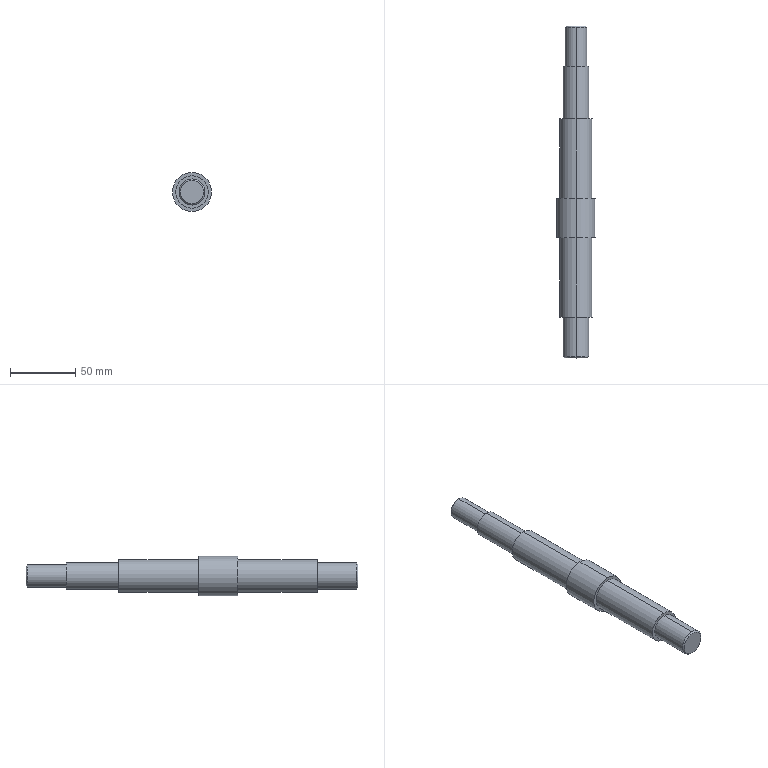Part | STEP file | PN_0021 | 1 solid | 23 faces | box 30 x 255 x 30 mm | volume 110798 mm3 | cylinder 12 | plane 7 | cone 4 | commonest cylinder face diameters 20 x4 25 x4 17 x2 30 x2
STEP:
#1=CARTESIAN_POINT('',(0.,0.,0.));
#2=DIRECTION('',(0.,0.,1.));
#3=DIRECTION('',(1.,0.,0.));
#4=AXIS2_PLACEMENT_3D('',#1,#2,#3);
#5=CARTESIAN_POINT('',(0.,255.,7.5));
#6=VERTEX_POINT('',#5);
#7=CARTESIAN_POINT('',(0.,255.,-7.5));
#8=VERTEX_POINT('',#7);
#9=CARTESIAN_POINT('',(0.,255.,0.));
#10=DIRECTION('',(0.,1.,0.));
#11=DIRECTION('',(0.,0.,1.));
#12=AXIS2_PLACEMENT_3D('',#9,#10,#11);
#13=CIRCLE('',#12,7.5);
#14=CARTESIAN_POINT('',(0.,254.,0.));
#15=DIRECTION('',(0.,-1.,0.));
#16=DIRECTION('',(0.,0.,-1.));
#17=AXIS2_PLACEMENT_3D('',#14,#15,#16);
#18=CONICAL_SURFACE('',#17,8.5,0.7854);
#19=CARTESIAN_POINT('',(3.142,-1.));
#20=DIRECTION('',(-1.,0.));
#21=VECTOR('',#20,1.);
#22=LINE('',#19,#21);
#23=(GEOMETRIC_REPRESENTATION_CONTEXT(2)PARAMETRIC_REPRESENTATION_CONTEXT()REPRESENTATION_CONTEXT('',''));
#24=DEFINITIONAL_REPRESENTATION('',(#22),#23);
#25=PCURVE('',#18,#24);
#26=CARTESIAN_POINT('',(0.,255.,0.));
#27=DIRECTION('',(0.,1.,0.));
#28=DIRECTION('',(0.,0.,1.));
#29=AXIS2_PLACEMENT_3D('',#26,#27,#28);
#30=PLANE('',#29);
#31=CARTESIAN_POINT('',(0.,0.));
#32=DIRECTION('',(1.,0.));
#33=AXIS2_PLACEMENT_2D('',#31,#32);
#34=CIRCLE('',#33,7.5);
#35=(GEOMETRIC_REPRESENTATION_CONTEXT(2)PARAMETRIC_REPRESENTATION_CONTEXT()REPRESENTATION_CONTEXT('',''));
#36=DEFINITIONAL_REPRESENTATION('',(#34),#35);
#37=PCURVE('',#30,#36);
#38=SURFACE_CURVE('',#13,(#25,#37),.PCURVE_S1.);
#39=EDGE_CURVE('',#6,#8,#38,.T.);
#40=ORIENTED_EDGE('',*,*,#39,.F.);
#41=CARTESIAN_POINT('',(0.,254.,8.5));
#42=VERTEX_POINT('',#41);
#43=CARTESIAN_POINT('',(0.,254.,8.5));
#44=DIRECTION('',(0.,-0.7071,0.7071));
#45=VECTOR('',#44,1.);
#46=LINE('',#43,#45);
#47=CARTESIAN_POINT('',(3.142,0.));
#48=DIRECTION('',(0.,1.));
#49=VECTOR('',#48,1.);
#50=LINE('',#47,#49);
#51=(GEOMETRIC_REPRESENTATION_CONTEXT(2)PARAMETRIC_REPRESENTATION_CONTEXT()REPRESENTATION_CONTEXT('',''));
#52=DEFINITIONAL_REPRESENTATION('',(#50),#51);
#53=PCURVE('',#18,#52);
#54=CARTESIAN_POINT('',(0.,254.,0.));
#55=DIRECTION('',(0.,-1.,0.));
#56=DIRECTION('',(0.,0.,-1.));
#57=AXIS2_PLACEMENT_3D('',#54,#55,#56);
#58=CONICAL_SURFACE('',#57,8.5,0.7854);
#59=CARTESIAN_POINT('',(3.142,0.));
#60=DIRECTION('',(0.,1.));
#61=VECTOR('',#60,1.);
#62=LINE('',#59,#61);
#63=(GEOMETRIC_REPRESENTATION_CONTEXT(2)PARAMETRIC_REPRESENTATION_CONTEXT()REPRESENTATION_CONTEXT('',''));
#64=DEFINITIONAL_REPRESENTATION('',(#62),#63);
#65=PCURVE('',#58,#64);
#66=SURFACE_CURVE('',#46,(#53,#65),.PCURVE_S1.);
#67=EDGE_CURVE('',#6,#42,#66,.T.);
#68=ORIENTED_EDGE('',*,*,#67,.T.);
#69=CARTESIAN_POINT('',(0.,254.,-8.5));
#70=VERTEX_POINT('',#69);
#71=CARTESIAN_POINT('',(0.,254.,0.));
#72=DIRECTION('',(0.,-1.,0.));
#73=DIRECTION('',(0.,0.,1.));
#74=AXIS2_PLACEMENT_3D('',#71,#72,#73);
#75=CIRCLE('',#74,8.5);
#76=CARTESIAN_POINT('',(-3.142,0.));
#77=DIRECTION('',(1.,0.));
#78=VECTOR('',#77,1.);
#79=LINE('',#76,#78);
#80=(GEOMETRIC_REPRESENTATION_CONTEXT(2)PARAMETRIC_REPRESENTATION_CONTEXT()REPRESENTATION_CONTEXT('',''));
#81=DEFINITIONAL_REPRESENTATION('',(#79),#80);
#82=PCURVE('',#18,#81);
#83=CARTESIAN_POINT('',(0.,0.,0.));
#84=DIRECTION('',(0.,-1.,0.));
#85=DIRECTION('',(0.,0.,-1.));
#86=AXIS2_PLACEMENT_3D('',#83,#84,#85);
#87=CYLINDRICAL_SURFACE('',#86,8.5);
#88=CARTESIAN_POINT('',(-3.142,-254.));
#89=DIRECTION('',(1.,0.));
#90=VECTOR('',#89,1.);
#91=LINE('',#88,#90);
#92=(GEOMETRIC_REPRESENTATION_CONTEXT(2)PARAMETRIC_REPRESENTATION_CONTEXT()REPRESENTATION_CONTEXT('',''));
#93=DEFINITIONAL_REPRESENTATION('',(#91),#92);
#94=PCURVE('',#87,#93);
#95=SURFACE_CURVE('',#75,(#82,#94),.PCURVE_S1.);
#96=EDGE_CURVE('',#70,#42,#95,.T.);
#97=ORIENTED_EDGE('',*,*,#96,.F.);
#98=CARTESIAN_POINT('',(0.,254.,-8.5));
#99=DIRECTION('',(0.,-0.7071,-0.7071));
#100=VECTOR('',#99,1.);
#101=LINE('',#98,#100);
#102=CARTESIAN_POINT('',(0.,0.));
#103=DIRECTION('',(0.,1.));
#104=VECTOR('',#103,1.);
#105=LINE('',#102,#104);
#106=(GEOMETRIC_REPRESENTATION_CONTEXT(2)PARAMETRIC_REPRESENTATION_CONTEXT()REPRESENTATION_CONTEXT('',''));
#107=DEFINITIONAL_REPRESENTATION('',(#105),#106);
#108=PCURVE('',#18,#107);
#109=CARTESIAN_POINT('',(6.283,0.));
#110=DIRECTION('',(0.,1.));
#111=VECTOR('',#110,1.);
#112=LINE('',#109,#111);
#113=(GEOMETRIC_REPRESENTATION_CONTEXT(2)PARAMETRIC_REPRESENTATION_CONTEXT()REPRESENTATION_CONTEXT('',''));
#114=DEFINITIONAL_REPRESENTATION('',(#112),#113);
#115=PCURVE('',#58,#114);
#116=SURFACE_CURVE('',#101,(#108,#115),.PCURVE_S1.);
#117=EDGE_CURVE('',#8,#70,#116,.T.);
#118=ORIENTED_EDGE('',*,*,#117,.F.);
#119=EDGE_LOOP('',(#40,#68,#97,#118));
#120=FACE_BOUND('',#119,.T.);
#121=ADVANCED_FACE('',(#120),#18,.T.);
#122=CARTESIAN_POINT('',(0.,0.,-9.));
#123=VERTEX_POINT('',#122);
#124=CARTESIAN_POINT('',(0.,0.,9.));
#125=VERTEX_POINT('',#124);
#126=CARTESIAN_POINT('',(0.,0.,0.));
#127=DIRECTION('',(0.,-1.,0.));
#128=DIRECTION('',(0.,0.,-1.));
#129=AXIS2_PLACEMENT_3D('',#126,#127,#128);
#130=CIRCLE('',#129,9.);
#131=CARTESIAN_POINT('',(0.,0.,0.));
#132=DIRECTION('',(0.,1.,0.));
#133=DIRECTION('',(0.,0.,1.));
#134=AXIS2_PLACEMENT_3D('',#131,#132,#133);
#135=CONICAL_SURFACE('',#134,9.,0.7854);
#136=CARTESIAN_POINT('',(3.142,0.));
#137=DIRECTION('',(-1.,0.));
#138=VECTOR('',#137,1.);
#139=LINE('',#136,#138);
#140=(GEOMETRIC_REPRESENTATION_CONTEXT(2)PARAMETRIC_REPRESENTATION_CONTEXT()REPRESENTATION_CONTEXT('',''));
#141=DEFINITIONAL_REPRESENTATION('',(#139),#140);
#142=PCURVE('',#135,#141);
#143=CARTESIAN_POINT('',(0.,0.,0.));
#144=DIRECTION('',(0.,-1.,0.));
#145=DIRECTION('',(0.,0.,-1.));
#146=AXIS2_PLACEMENT_3D('',#143,#144,#145);
#147=PLANE('',#146);
#148=CARTESIAN_POINT('',(0.,0.));
#149=DIRECTION('',(1.,0.));
#150=AXIS2_PLACEMENT_2D('',#148,#149);
#151=CIRCLE('',#150,9.);
#152=(GEOMETRIC_REPRESENTATION_CONTEXT(2)PARAMETRIC_REPRESENTATION_CONTEXT()REPRESENTATION_CONTEXT('',''));
#153=DEFINITIONAL_REPRESENTATION('',(#151),#152);
#154=PCURVE('',#147,#153);
#155=SURFACE_CURVE('',#130,(#142,#154),.PCURVE_S1.);
#156=EDGE_CURVE('',#123,#125,#155,.T.);
#157=ORIENTED_EDGE('',*,*,#156,.F.);
#158=CARTESIAN_POINT('',(0.,1.,-10.));
#159=VERTEX_POINT('',#158);
#160=CARTESIAN_POINT('',(0.,0.,-9.));
#161=DIRECTION('',(0.,0.7071,-0.7071));
#162=VECTOR('',#161,1.);
#163=LINE('',#160,#162);
#164=CARTESIAN_POINT('',(3.142,0.));
#165=DIRECTION('',(0.,1.));
#166=VECTOR('',#165,1.);
#167=LINE('',#164,#166);
#168=(GEOMETRIC_REPRESENTATION_CONTEXT(2)PARAMETRIC_REPRESENTATION_CONTEXT()REPRESENTATION_CONTEXT('',''));
#169=DEFINITIONAL_REPRESENTATION('',(#167),#168);
#170=PCURVE('',#135,#169);
#171=CARTESIAN_POINT('',(0.,0.,0.));
#172=DIRECTION('',(0.,1.,0.));
#173=DIRECTION('',(0.,0.,1.));
#174=AXIS2_PLACEMENT_3D('',#171,#172,#173);
#175=CONICAL_SURFACE('',#174,9.,0.7854);
#176=CARTESIAN_POINT('',(3.142,0.));
#177=DIRECTION('',(0.,1.));
#178=VECTOR('',#177,1.);
#179=LINE('',#176,#178);
#180=(GEOMETRIC_REPRESENTATION_CONTEXT(2)PARAMETRIC_REPRESENTATION_CONTEXT()REPRESENTATION_CONTEXT('',''));
#181=DEFINITIONAL_REPRESENTATION('',(#179),#180);
#182=PCURVE('',#175,#181);
#183=SURFACE_CURVE('',#163,(#170,#182),.PCURVE_S1.);
#184=EDGE_CURVE('',#123,#159,#183,.T.);
#185=ORIENTED_EDGE('',*,*,#184,.T.);
#186=CARTESIAN_POINT('',(0.,1.,10.));
#187=VERTEX_POINT('',#186);
#188=CARTESIAN_POINT('',(0.,1.,0.));
#189=DIRECTION('',(0.,1.,0.));
#190=DIRECTION('',(0.,0.,-1.));
#191=AXIS2_PLACEMENT_3D('',#188,#189,#190);
#192=CIRCLE('',#191,10.);
#193=CARTESIAN_POINT('',(-3.142,1.));
#194=DIRECTION('',(1.,0.));
#195=VECTOR('',#194,1.);
#196=LINE('',#193,#195);
#197=(GEOMETRIC_REPRESENTATION_CONTEXT(2)PARAMETRIC_REPRESENTATION_CONTEXT()REPRESENTATION_CONTEXT('',''));
#198=DEFINITIONAL_REPRESENTATION('',(#196),#197);
#199=PCURVE('',#135,#198);
#200=CARTESIAN_POINT('',(0.,0.,0.));
#201=DIRECTION('',(0.,-1.,0.));
#202=DIRECTION('',(0.,0.,-1.));
#203=AXIS2_PLACEMENT_3D('',#200,#201,#202);
#204=CYLINDRICAL_SURFACE('',#203,10.);
#205=CARTESIAN_POINT('',(6.283,-1.));
#206=DIRECTION('',(-1.,0.));
#207=VECTOR('',#206,1.);
#208=LINE('',#205,#207);
#209=(GEOMETRIC_REPRESENTATION_CONTEXT(2)PARAMETRIC_REPRESENTATION_CONTEXT()REPRESENTATION_CONTEXT('',''));
#210=DEFINITIONAL_REPRESENTATION('',(#208),#209);
#211=PCURVE('',#204,#210);
#212=SURFACE_CURVE('',#192,(#199,#211),.PCURVE_S1.);
#213=EDGE_CURVE('',#187,#159,#212,.T.);
#214=ORIENTED_EDGE('',*,*,#213,.F.);
#215=CARTESIAN_POINT('',(0.,0.,9.));
#216=DIRECTION('',(0.,0.7071,0.7071));
#217=VECTOR('',#216,1.);
#218=LINE('',#215,#217);
#219=CARTESIAN_POINT('',(0.,0.));
#220=DIRECTION('',(0.,1.));
#221=VECTOR('',#220,1.);
#222=LINE('',#219,#221);
#223=(GEOMETRIC_REPRESENTATION_CONTEXT(2)PARAMETRIC_REPRESENTATION_CONTEXT()REPRESENTATION_CONTEXT('',''));
#224=DEFINITIONAL_REPRESENTATION('',(#222),#223);
#225=PCURVE('',#135,#224);
#226=CARTESIAN_POINT('',(6.283,0.));
#227=DIRECTION('',(0.,1.));
#228=VECTOR('',#227,1.);
#229=LINE('',#226,#228);
#230=(GEOMETRIC_REPRESENTATION_CONTEXT(2)PARAMETRIC_REPRESENTATION_CONTEXT()REPRESENTATION_CONTEXT('',''));
#231=DEFINITIONAL_REPRESENTATION('',(#229),#230);
#232=PCURVE('',#175,#231);
#233=SURFACE_CURVE('',#218,(#225,#232),.PCURVE_S1.);
#234=EDGE_CURVE('',#125,#187,#233,.T.);
#235=ORIENTED_EDGE('',*,*,#234,.F.);
#236=EDGE_LOOP('',(#157,#185,#214,#235));
#237=FACE_BOUND('',#236,.T.);
#238=ADVANCED_FACE('',(#237),#135,.T.);
#239=CARTESIAN_POINT('',(0.,31.2,-10.));
#240=VERTEX_POINT('',#239);
#241=CARTESIAN_POINT('',(0.,31.2,10.));
#242=VERTEX_POINT('',#241);
#243=CARTESIAN_POINT('',(0.,31.2,0.));
#244=DIRECTION('',(0.,-1.,0.));
#245=DIRECTION('',(0.,0.,-1.));
#246=AXIS2_PLACEMENT_3D('',#243,#244,#245);
#247=CIRCLE('',#246,10.);
#248=CARTESIAN_POINT('',(0.,-31.2));
#249=DIRECTION('',(1.,0.));
#250=VECTOR('',#249,1.);
#251=LINE('',#248,#250);
#252=(GEOMETRIC_REPRESENTATION_CONTEXT(2)PARAMETRIC_REPRESENTATION_CONTEXT()REPRESENTATION_CONTEXT('',''));
#253=DEFINITIONAL_REPRESENTATION('',(#251),#252);
#254=PCURVE('',#204,#253);
#255=CARTESIAN_POINT('',(10.,31.2,0.));
#256=DIRECTION('',(0.,-1.,0.));
#257=DIRECTION('',(0.,0.,-1.));
#258=AXIS2_PLACEMENT_3D('',#255,#256,#257);
#259=PLANE('',#258);
#260=CARTESIAN_POINT('',(0.,-10.));
#261=DIRECTION('',(1.,0.));
#262=AXIS2_PLACEMENT_2D('',#260,#261);
#263=CIRCLE('',#262,10.);
#264=(GEOMETRIC_REPRESENTATION_CONTEXT(2)PARAMETRIC_REPRESENTATION_CONTEXT()REPRESENTATION_CONTEXT('',''));
#265=DEFINITIONAL_REPRESENTATION('',(#263),#264);
#266=PCURVE('',#259,#265);
#267=SURFACE_CURVE('',#247,(#254,#266),.PCURVE_S1.);
#268=EDGE_CURVE('',#240,#242,#267,.T.);
#269=ORIENTED_EDGE('',*,*,#268,.T.);
#270=CARTESIAN_POINT('',(0.,0.,10.));
#271=DIRECTION('',(0.,-1.,0.));
#272=VECTOR('',#271,1.);
#273=LINE('',#270,#272);
#274=CARTESIAN_POINT('',(3.142,0.));
#275=DIRECTION('',(0.,1.));
#276=VECTOR('',#275,1.);
#277=LINE('',#274,#276);
#278=(GEOMETRIC_REPRESENTATION_CONTEXT(2)PARAMETRIC_REPRESENTATION_CONTEXT()REPRESENTATION_CONTEXT('',''));
#279=DEFINITIONAL_REPRESENTATION('',(#277),#278);
#280=PCURVE('',#204,#279);
#281=CARTESIAN_POINT('',(0.,0.,0.));
#282=DIRECTION('',(0.,-1.,0.));
#283=DIRECTION('',(0.,0.,-1.));
#284=AXIS2_PLACEMENT_3D('',#281,#282,#283);
#285=CYLINDRICAL_SURFACE('',#284,10.);
#286=CARTESIAN_POINT('',(3.142,0.));
#287=DIRECTION('',(0.,1.));
#288=VECTOR('',#287,1.);
#289=LINE('',#286,#288);
#290=(GEOMETRIC_REPRESENTATION_CONTEXT(2)PARAMETRIC_REPRESENTATION_CONTEXT()REPRESENTATION_CONTEXT('',''));
#291=DEFINITIONAL_REPRESENTATION('',(#289),#290);
#292=PCURVE('',#285,#291);
#293=SURFACE_CURVE('',#273,(#280,#292),.PCURVE_S1.);
#294=EDGE_CURVE('',#242,#187,#293,.T.);
#295=ORIENTED_EDGE('',*,*,#294,.T.);
#296=ORIENTED_EDGE('',*,*,#213,.T.);
#297=CARTESIAN_POINT('',(0.,0.,-10.));
#298=DIRECTION('',(0.,-1.,0.));
#299=VECTOR('',#298,1.);
#300=LINE('',#297,#299);
#301=CARTESIAN_POINT('',(0.,0.));
#302=DIRECTION('',(0.,1.));
#303=VECTOR('',#302,1.);
#304=LINE('',#301,#303);
#305=(GEOMETRIC_REPRESENTATION_CONTEXT(2)PARAMETRIC_REPRESENTATION_CONTEXT()REPRESENTATION_CONTEXT('',''));
#306=DEFINITIONAL_REPRESENTATION('',(#304),#305);
#307=PCURVE('',#204,#306);
#308=CARTESIAN_POINT('',(6.283,0.));
#309=DIRECTION('',(0.,1.));
#310=VECTOR('',#309,1.);
#311=LINE('',#308,#310);
#312=(GEOMETRIC_REPRESENTATION_CONTEXT(2)PARAMETRIC_REPRESENTATION_CONTEXT()REPRESENTATION_CONTEXT('',''));
#313=DEFINITIONAL_REPRESENTATION('',(#311),#312);
#314=PCURVE('',#285,#313);
#315=SURFACE_CURVE('',#300,(#307,#314),.PCURVE_S1.);
#316=EDGE_CURVE('',#240,#159,#315,.T.);
#317=ORIENTED_EDGE('',*,*,#316,.F.);
#318=EDGE_LOOP('',(#269,#295,#296,#317));
#319=FACE_BOUND('',#318,.T.);
#320=ADVANCED_FACE('',(#319),#204,.T.);
#321=CARTESIAN_POINT('',(0.,92.5,-12.5));
#322=VERTEX_POINT('',#321);
#323=CARTESIAN_POINT('',(0.,92.5,12.5));
#324=VERTEX_POINT('',#323);
#325=CARTESIAN_POINT('',(0.,92.5,0.));
#326=DIRECTION('',(0.,-1.,0.));
#327=DIRECTION('',(0.,0.,-1.));
#328=AXIS2_PLACEMENT_3D('',#325,#326,#327);
#329=CIRCLE('',#328,12.5);
#330=CARTESIAN_POINT('',(0.,0.,0.));
#331=DIRECTION('',(0.,-1.,0.));
#332=DIRECTION('',(0.,0.,-1.));
#333=AXIS2_PLACEMENT_3D('',#330,#331,#332);
#334=CYLINDRICAL_SURFACE('',#333,12.5);
#335=CARTESIAN_POINT('',(0.,-92.5));
#336=DIRECTION('',(1.,0.));
#337=VECTOR('',#336,1.);
#338=LINE('',#335,#337);
#339=(GEOMETRIC_REPRESENTATION_CONTEXT(2)PARAMETRIC_REPRESENTATION_CONTEXT()REPRESENTATION_CONTEXT('',''));
#340=DEFINITIONAL_REPRESENTATION('',(#338),#339);
#341=PCURVE('',#334,#340);
#342=CARTESIAN_POINT('',(12.5,92.5,0.));
#343=DIRECTION('',(0.,-1.,0.));
#344=DIRECTION('',(0.,0.,-1.));
#345=AXIS2_PLACEMENT_3D('',#342,#343,#344);
#346=PLANE('',#345);
#347=CARTESIAN_POINT('',(0.,-12.5));
#348=DIRECTION('',(1.,0.));
#349=AXIS2_PLACEMENT_2D('',#347,#348);
#350=CIRCLE('',#349,12.5);
#351=(GEOMETRIC_REPRESENTATION_CONTEXT(2)PARAMETRIC_REPRESENTATION_CONTEXT()REPRESENTATION_CONTEXT('',''));
#352=DEFINITIONAL_REPRESENTATION('',(#350),#351);
#353=PCURVE('',#346,#352);
#354=SURFACE_CURVE('',#329,(#341,#353),.PCURVE_S1.);
#355=EDGE_CURVE('',#322,#324,#354,.T.);
#356=ORIENTED_EDGE('',*,*,#355,.T.);
#357=CARTESIAN_POINT('',(0.,31.2,12.5));
#358=VERTEX_POINT('',#357);
#359=CARTESIAN_POINT('',(0.,0.,12.5));
#360=DIRECTION('',(0.,-1.,0.));
#361=VECTOR('',#360,1.);
#362=LINE('',#359,#361);
#363=CARTESIAN_POINT('',(3.142,0.));
#364=DIRECTION('',(0.,1.));
#365=VECTOR('',#364,1.);
#366=LINE('',#363,#365);
#367=(GEOMETRIC_REPRESENTATION_CONTEXT(2)PARAMETRIC_REPRESENTATION_CONTEXT()REPRESENTATION_CONTEXT('',''));
#368=DEFINITIONAL_REPRESENTATION('',(#366),#367);
#369=PCURVE('',#334,#368);
#370=CARTESIAN_POINT('',(0.,0.,0.));
#371=DIRECTION('',(0.,-1.,0.));
#372=DIRECTION('',(0.,0.,-1.));
#373=AXIS2_PLACEMENT_3D('',#370,#371,#372);
#374=CYLINDRICAL_SURFACE('',#373,12.5);
#375=CARTESIAN_POINT('',(3.142,0.));
#376=DIRECTION('',(0.,1.));
#377=VECTOR('',#376,1.);
#378=LINE('',#375,#377);
#379=(GEOMETRIC_REPRESENTATION_CONTEXT(2)PARAMETRIC_REPRESENTATION_CONTEXT()REPRESENTATION_CONTEXT('',''));
#380=DEFINITIONAL_REPRESENTATION('',(#378),#379);
#381=PCURVE('',#374,#380);
#382=SURFACE_CURVE('',#362,(#369,#381),.PCURVE_S1.);
#383=EDGE_CURVE('',#324,#358,#382,.T.);
#384=ORIENTED_EDGE('',*,*,#383,.T.);
#385=CARTESIAN_POINT('',(0.,31.2,-12.5));
#386=VERTEX_POINT('',#385);
#387=CARTESIAN_POINT('',(0.,31.2,0.));
#388=DIRECTION('',(0.,-1.,0.));
#389=DIRECTION('',(0.,0.,-1.));
#390=AXIS2_PLACEMENT_3D('',#387,#388,#389);
#391=CIRCLE('',#390,12.5);
#392=CARTESIAN_POINT('',(0.,-31.2));
#393=DIRECTION('',(1.,0.));
#394=VECTOR('',#393,1.);
#395=LINE('',#392,#394);
#396=(GEOMETRIC_REPRESENTATION_CONTEXT(2)PARAMETRIC_REPRESENTATION_CONTEXT()REPRESENTATION_CONTEXT('',''));
#397=DEFINITIONAL_REPRESENTATION('',(#395),#396);
#398=PCURVE('',#334,#397);
#399=CARTESIAN_POINT('',(0.,-10.));
#400=DIRECTION('',(1.,0.));
#401=AXIS2_PLACEMENT_2D('',#399,#400);
#402=CIRCLE('',#401,12.5);
#403=(GEOMETRIC_REPRESENTATION_CONTEXT(2)PARAMETRIC_REPRESENTATION_CONTEXT()REPRESENTATION_CONTEXT('',''));
#404=DEFINITIONAL_REPRESENTATION('',(#402),#403);
#405=PCURVE('',#259,#404);
#406=SURFACE_CURVE('',#391,(#398,#405),.PCURVE_S1.);
#407=EDGE_CURVE('',#386,#358,#406,.T.);
#408=ORIENTED_EDGE('',*,*,#407,.F.);
#409=CARTESIAN_POINT('',(0.,0.,-12.5));
#410=DIRECTION('',(0.,-1.,0.));
#411=VECTOR('',#410,1.);
#412=LINE('',#409,#411);
#413=CARTESIAN_POINT('',(0.,0.));
#414=DIRECTION('',(0.,1.));
#415=VECTOR('',#414,1.);
#416=LINE('',#413,#415);
#417=(GEOMETRIC_REPRESENTATION_CONTEXT(2)PARAMETRIC_REPRESENTATION_CONTEXT()REPRESENTATION_CONTEXT('',''));
#418=DEFINITIONAL_REPRESENTATION('',(#416),#417);
#419=PCURVE('',#334,#418);
#420=CARTESIAN_POINT('',(6.283,0.));
#421=DIRECTION('',(0.,1.));
#422=VECTOR('',#421,1.);
#423=LINE('',#420,#422);
#424=(GEOMETRIC_REPRESENTATION_CONTEXT(2)PARAMETRIC_REPRESENTATION_CONTEXT()REPRESENTATION_CONTEXT('',''));
#425=DEFINITIONAL_REPRESENTATION('',(#423),#424);
#426=PCURVE('',#374,#425);
#427=SURFACE_CURVE('',#412,(#419,#426),.PCURVE_S1.);
#428=EDGE_CURVE('',#322,#386,#427,.T.);
#429=ORIENTED_EDGE('',*,*,#428,.F.);
#430=EDGE_LOOP('',(#356,#384,#408,#429));
#431=FACE_BOUND('',#430,.T.);
#432=ADVANCED_FACE('',(#431),#334,.T.);
#433=CARTESIAN_POINT('',(0.,122.5,-15.));
#434=VERTEX_POINT('',#433);
#435=CARTESIAN_POINT('',(0.,122.5,15.));
#436=VERTEX_POINT('',#435);
#437=CARTESIAN_POINT('',(0.,122.5,0.));
#438=DIRECTION('',(0.,-1.,0.));
#439=DIRECTION('',(0.,0.,-1.));
#440=AXIS2_PLACEMENT_3D('',#437,#438,#439);
#441=CIRCLE('',#440,15.);
#442=CARTESIAN_POINT('',(0.,0.,0.));
#443=DIRECTION('',(0.,-1.,0.));
#444=DIRECTION('',(0.,0.,-1.));
#445=AXIS2_PLACEMENT_3D('',#442,#443,#444);
#446=CYLINDRICAL_SURFACE('',#445,15.);
#447=CARTESIAN_POINT('',(0.,-122.5));
#448=DIRECTION('',(1.,0.));
#449=VECTOR('',#448,1.);
#450=LINE('',#447,#449);
#451=(GEOMETRIC_REPRESENTATION_CONTEXT(2)PARAMETRIC_REPRESENTATION_CONTEXT()REPRESENTATION_CONTEXT('',''));
#452=DEFINITIONAL_REPRESENTATION('',(#450),#451);
#453=PCURVE('',#446,#452);
#454=CARTESIAN_POINT('',(12.5,122.5,0.));
#455=DIRECTION('',(0.,1.,0.));
#456=DIRECTION('',(0.,0.,1.));
#457=AXIS2_PLACEMENT_3D('',#454,#455,#456);
#458=PLANE('',#457);
#459=CARTESIAN_POINT('',(-15.,-12.5));
#460=CARTESIAN_POINT('',(-15.,13.481));
#461=CARTESIAN_POINT('',(7.5,0.4904));
#462=CARTESIAN_POINT('',(30.,-12.5));
#463=CARTESIAN_POINT('',(7.5,-25.49));
#464=CARTESIAN_POINT('',(-15.,-38.481));
#465=CARTESIAN_POINT('',(-15.,-12.5));
#466=(BOUNDED_CURVE()B_SPLINE_CURVE(2,(#459,#460,#461,#462,#463,#464,#465),.UNSPECIFIED.,.T.,.F.)B_SPLINE_CURVE_WITH_KNOTS((1,2,2,2,2,1),(-2.094,0.,2.094,4.189,6.283,8.378),.UNSPECIFIED.)CURVE()GEOMETRIC_REPRESENTATION_ITEM()RATIONAL_B_SPLINE_CURVE((1.,0.5,1.,0.5,1.,0.5,1.))REPRESENTATION_ITEM(''));
#467=(GEOMETRIC_REPRESENTATION_CONTEXT(2)PARAMETRIC_REPRESENTATION_CONTEXT()REPRESENTATION_CONTEXT('',''));
#468=DEFINITIONAL_REPRESENTATION('',(#466),#467);
#469=PCURVE('',#458,#468);
#470=SURFACE_CURVE('',#441,(#453,#469),.PCURVE_S1.);
#471=EDGE_CURVE('',#434,#436,#470,.T.);
#472=ORIENTED_EDGE('',*,*,#471,.T.);
#473=CARTESIAN_POINT('',(0.,92.5,15.));
#474=VERTEX_POINT('',#473);
#475=CARTESIAN_POINT('',(0.,0.,15.));
#476=DIRECTION('',(0.,-1.,0.));
#477=VECTOR('',#476,1.);
#478=LINE('',#475,#477);
#479=CARTESIAN_POINT('',(3.142,0.));
#480=DIRECTION('',(0.,1.));
#481=VECTOR('',#480,1.);
#482=LINE('',#479,#481);
#483=(GEOMETRIC_REPRESENTATION_CONTEXT(2)PARAMETRIC_REPRESENTATION_CONTEXT()REPRESENTATION_CONTEXT('',''));
#484=DEFINITIONAL_REPRESENTATION('',(#482),#483);
#485=PCURVE('',#446,#484);
#486=CARTESIAN_POINT('',(0.,0.,0.));
#487=DIRECTION('',(0.,-1.,0.));
#488=DIRECTION('',(0.,0.,-1.));
#489=AXIS2_PLACEMENT_3D('',#486,#487,#488);
#490=CYLINDRICAL_SURFACE('',#489,15.);
#491=CARTESIAN_POINT('',(3.142,0.));
#492=DIRECTION('',(0.,1.));
#493=VECTOR('',#492,1.);
#494=LINE('',#491,#493);
#495=(GEOMETRIC_REPRESENTATION_CONTEXT(2)PARAMETRIC_REPRESENTATION_CONTEXT()REPRESENTATION_CONTEXT('',''));
#496=DEFINITIONAL_REPRESENTATION('',(#494),#495);
#497=PCURVE('',#490,#496);
#498=SURFACE_CURVE('',#478,(#485,#497),.PCURVE_S1.);
#499=EDGE_CURVE('',#436,#474,#498,.T.);
#500=ORIENTED_EDGE('',*,*,#499,.T.);
#501=CARTESIAN_POINT('',(0.,92.5,-15.));
#502=VERTEX_POINT('',#501);
#503=CARTESIAN_POINT('',(0.,92.5,0.));
#504=DIRECTION('',(0.,-1.,0.));
#505=DIRECTION('',(0.,0.,-1.));
#506=AXIS2_PLACEMENT_3D('',#503,#504,#505);
#507=CIRCLE('',#506,15.);
#508=CARTESIAN_POINT('',(0.,-92.5));
#509=DIRECTION('',(1.,0.));
#510=VECTOR('',#509,1.);
#511=LINE('',#508,#510);
#512=(GEOMETRIC_REPRESENTATION_CONTEXT(2)PARAMETRIC_REPRESENTATION_CONTEXT()REPRESENTATION_CONTEXT('',''));
#513=DEFINITIONAL_REPRESENTATION('',(#511),#512);
#514=PCURVE('',#446,#513);
#515=CARTESIAN_POINT('',(0.,-12.5));
#516=DIRECTION('',(1.,0.));
#517=AXIS2_PLACEMENT_2D('',#515,#516);
#518=CIRCLE('',#517,15.);
#519=(GEOMETRIC_REPRESENTATION_CONTEXT(2)PARAMETRIC_REPRESENTATION_CONTEXT()REPRESENTATION_CONTEXT('',''));
#520=DEFINITIONAL_REPRESENTATION('',(#518),#519);
#521=PCURVE('',#346,#520);
#522=SURFACE_CURVE('',#507,(#514,#521),.PCURVE_S1.);
#523=EDGE_CURVE('',#502,#474,#522,.T.);
#524=ORIENTED_EDGE('',*,*,#523,.F.);
#525=CARTESIAN_POINT('',(0.,0.,-15.));
#526=DIRECTION('',(0.,-1.,0.));
#527=VECTOR('',#526,1.);
#528=LINE('',#525,#527);
#529=CARTESIAN_POINT('',(0.,0.));
#530=DIRECTION('',(0.,1.));
#531=VECTOR('',#530,1.);
#532=LINE('',#529,#531);
#533=(GEOMETRIC_REPRESENTATION_CONTEXT(2)PARAMETRIC_REPRESENTATION_CONTEXT()REPRESENTATION_CONTEXT('',''));
#534=DEFINITIONAL_REPRESENTATION('',(#532),#533);
#535=PCURVE('',#446,#534);
#536=CARTESIAN_POINT('',(6.283,0.));
#537=DIRECTION('',(0.,1.));
#538=VECTOR('',#537,1.);
#539=LINE('',#536,#538);
#540=(GEOMETRIC_REPRESENTATION_CONTEXT(2)PARAMETRIC_REPRESENTATION_CONTEXT()REPRESENTATION_CONTEXT('',''));
#541=DEFINITIONAL_REPRESENTATION('',(#539),#540);
#542=PCURVE('',#490,#541);
#543=SURFACE_CURVE('',#528,(#535,#542),.PCURVE_S1.);
#544=EDGE_CURVE('',#434,#502,#543,.T.);
#545=ORIENTED_EDGE('',*,*,#544,.F.);
#546=EDGE_LOOP('',(#472,#500,#524,#545));
#547=FACE_BOUND('',#546,.T.);
#548=ADVANCED_FACE('',(#547),#446,.T.);
#549=CARTESIAN_POINT('',(0.,183.8,-12.5));
#550=VERTEX_POINT('',#549);
#551=CARTESIAN_POINT('',(0.,183.8,12.5));
#552=VERTEX_POINT('',#551);
#553=CARTESIAN_POINT('',(0.,183.8,0.));
#554=DIRECTION('',(0.,-1.,0.));
#555=DIRECTION('',(0.,0.,-1.));
#556=AXIS2_PLACEMENT_3D('',#553,#554,#555);
#557=CIRCLE('',#556,12.5);
#558=CARTESIAN_POINT('',(0.,0.,0.));
#559=DIRECTION('',(0.,-1.,0.));
#560=DIRECTION('',(0.,0.,-1.));
#561=AXIS2_PLACEMENT_3D('',#558,#559,#560);
#562=CYLINDRICAL_SURFACE('',#561,12.5);
#563=CARTESIAN_POINT('',(0.,-183.8));
#564=DIRECTION('',(1.,0.));
#565=VECTOR('',#564,1.);
#566=LINE('',#563,#565);
#567=(GEOMETRIC_REPRESENTATION_CONTEXT(2)PARAMETRIC_REPRESENTATION_CONTEXT()REPRESENTATION_CONTEXT('',''));
#568=DEFINITIONAL_REPRESENTATION('',(#566),#567);
#569=PCURVE('',#562,#568);
#570=CARTESIAN_POINT('',(10.,183.8,0.));
#571=DIRECTION('',(0.,1.,0.));
#572=DIRECTION('',(0.,0.,1.));
#573=AXIS2_PLACEMENT_3D('',#570,#571,#572);
#574=PLANE('',#573);
#575=CARTESIAN_POINT('',(-12.5,-10.));
#576=CARTESIAN_POINT('',(-12.5,11.651));
#577=CARTESIAN_POINT('',(6.25,0.8253));
#578=CARTESIAN_POINT('',(25.,-10.));
#579=CARTESIAN_POINT('',(6.25,-20.825));
#580=CARTESIAN_POINT('',(-12.5,-31.651));
#581=CARTESIAN_POINT('',(-12.5,-10.));
#582=(BOUNDED_CURVE()B_SPLINE_CURVE(2,(#575,#576,#577,#578,#579,#580,#581),.UNSPECIFIED.,.T.,.F.)B_SPLINE_CURVE_WITH_KNOTS((1,2,2,2,2,1),(-2.094,0.,2.094,4.189,6.283,8.378),.UNSPECIFIED.)CURVE()GEOMETRIC_REPRESENTATION_ITEM()RATIONAL_B_SPLINE_CURVE((1.,0.5,1.,0.5,1.,0.5,1.))REPRESENTATION_ITEM(''));
#583=(GEOMETRIC_REPRESENTATION_CONTEXT(2)PARAMETRIC_REPRESENTATION_CONTEXT()REPRESENTATION_CONTEXT('',''));
#584=DEFINITIONAL_REPRESENTATION('',(#582),#583);
#585=PCURVE('',#574,#584);
#586=SURFACE_CURVE('',#557,(#569,#585),.PCURVE_S1.);
#587=EDGE_CURVE('',#550,#552,#586,.T.);
#588=ORIENTED_EDGE('',*,*,#587,.T.);
#589=CARTESIAN_POINT('',(0.,122.5,12.5));
#590=VERTEX_POINT('',#589);
#591=CARTESIAN_POINT('',(0.,0.,12.5));
#592=DIRECTION('',(0.,-1.,0.));
#593=VECTOR('',#592,1.);
#594=LINE('',#591,#593);
#595=CARTESIAN_POINT('',(3.142,0.));
#596=DIRECTION('',(0.,1.));
#597=VECTOR('',#596,1.);
#598=LINE('',#595,#597);
#599=(GEOMETRIC_REPRESENTATION_CONTEXT(2)PARAMETRIC_REPRESENTATION_CONTEXT()REPRESENTATION_CONTEXT('',''));
#600=DEFINITIONAL_REPRESENTATION('',(#598),#599);
#601=PCURVE('',#562,#600);
#602=CARTESIAN_POINT('',(0.,0.,0.));
#603=DIRECTION('',(0.,-1.,0.));
#604=DIRECTION('',(0.,0.,-1.));
#605=AXIS2_PLACEMENT_3D('',#602,#603,#604);
#606=CYLINDRICAL_SURFACE('',#605,12.5);
#607=CARTESIAN_POINT('',(3.142,0.));
#608=DIRECTION('',(0.,1.));
#609=VECTOR('',#608,1.);
#610=LINE('',#607,#609);
#611=(GEOMETRIC_REPRESENTATION_CONTEXT(2)PARAMETRIC_REPRESENTATION_CONTEXT()REPRESENTATION_CONTEXT('',''));
#612=DEFINITIONAL_REPRESENTATION('',(#610),#611);
#613=PCURVE('',#606,#612);
#614=SURFACE_CURVE('',#594,(#601,#613),.PCURVE_S1.);
#615=EDGE_CURVE('',#552,#590,#614,.T.);
#616=ORIENTED_EDGE('',*,*,#615,.T.);
#617=CARTESIAN_POINT('',(0.,122.5,-12.5));
#618=VERTEX_POINT('',#617);
#619=CARTESIAN_POINT('',(0.,122.5,0.));
#620=DIRECTION('',(0.,-1.,0.));
#621=DIRECTION('',(0.,0.,-1.));
#622=AXIS2_PLACEMENT_3D('',#619,#620,#621);
#623=CIRCLE('',#622,12.5);
#624=CARTESIAN_POINT('',(0.,-122.5));
#625=DIRECTION('',(1.,0.));
#626=VECTOR('',#625,1.);
#627=LINE('',#624,#626);
#628=(GEOMETRIC_REPRESENTATION_CONTEXT(2)PARAMETRIC_REPRESENTATION_CONTEXT()REPRESENTATION_CONTEXT('',''));
#629=DEFINITIONAL_REPRESENTATION('',(#627),#628);
#630=PCURVE('',#562,#629);
#631=CARTESIAN_POINT('',(-12.5,-12.5));
#632=CARTESIAN_POINT('',(-12.5,9.151));
#633=CARTESIAN_POINT('',(6.25,-1.675));
#634=CARTESIAN_POINT('',(25.,-12.5));
#635=CARTESIAN_POINT('',(6.25,-23.325));
#636=CARTESIAN_POINT('',(-12.5,-34.151));
#637=CARTESIAN_POINT('',(-12.5,-12.5));
#638=(BOUNDED_CURVE()B_SPLINE_CURVE(2,(#631,#632,#633,#634,#635,#636,#637),.UNSPECIFIED.,.T.,.F.)B_SPLINE_CURVE_WITH_KNOTS((1,2,2,2,2,1),(-2.094,0.,2.094,4.189,6.283,8.378),.UNSPECIFIED.)CURVE()GEOMETRIC_REPRESENTATION_ITEM()RATIONAL_B_SPLINE_CURVE((1.,0.5,1.,0.5,1.,0.5,1.))REPRESENTATION_ITEM(''));
#639=(GEOMETRIC_REPRESENTATION_CONTEXT(2)PARAMETRIC_REPRESENTATION_CONTEXT()REPRESENTATION_CONTEXT('',''));
#640=DEFINITIONAL_REPRESENTATION('',(#638),#639);
#641=PCURVE('',#458,#640);
#642=SURFACE_CURVE('',#623,(#630,#641),.PCURVE_S1.);
#643=EDGE_CURVE('',#618,#590,#642,.T.);
#644=ORIENTED_EDGE('',*,*,#643,.F.);
#645=CARTESIAN_POINT('',(0.,0.,-12.5));
#646=DIRECTION('',(0.,-1.,0.));
#647=VECTOR('',#646,1.);
#648=LINE('',#645,#647);
#649=CARTESIAN_POINT('',(0.,0.));
#650=DIRECTION('',(0.,1.));
#651=VECTOR('',#650,1.);
#652=LINE('',#649,#651);
#653=(GEOMETRIC_REPRESENTATION_CONTEXT(2)PARAMETRIC_REPRESENTATION_CONTEXT()REPRESENTATION_CONTEXT('',''));
#654=DEFINITIONAL_REPRESENTATION('',(#652),#653);
#655=PCURVE('',#562,#654);
#656=CARTESIAN_POINT('',(6.283,0.));
#657=DIRECTION('',(0.,1.));
#658=VECTOR('',#657,1.);
#659=LINE('',#656,#658);
#660=(GEOMETRIC_REPRESENTATION_CONTEXT(2)PARAMETRIC_REPRESENTATION_CONTEXT()REPRESENTATION_CONTEXT('',''));
#661=DEFINITIONAL_REPRESENTATION('',(#659),#660);
#662=PCURVE('',#606,#661);
#663=SURFACE_CURVE('',#648,(#655,#662),.PCURVE_S1.);
#664=EDGE_CURVE('',#550,#618,#663,.T.);
#665=ORIENTED_EDGE('',*,*,#664,.F.);
#666=EDGE_LOOP('',(#588,#616,#644,#665));
#667=FACE_BOUND('',#666,.T.);
#668=ADVANCED_FACE('',(#667),#562,.T.);
#669=CARTESIAN_POINT('',(0.,224.,-10.));
#670=VERTEX_POINT('',#669);
#671=CARTESIAN_POINT('',(0.,224.,10.));
#672=VERTEX_POINT('',#671);
#673=CARTESIAN_POINT('',(0.,224.,0.));
#674=DIRECTION('',(0.,-1.,0.));
#675=DIRECTION('',(0.,0.,-1.));
#676=AXIS2_PLACEMENT_3D('',#673,#674,#675);
#677=CIRCLE('',#676,10.);
#678=CARTESIAN_POINT('',(0.,0.,0.));
#679=DIRECTION('',(0.,-1.,0.));
#680=DIRECTION('',(0.,0.,-1.));
#681=AXIS2_PLACEMENT_3D('',#678,#679,#680);
#682=CYLINDRICAL_SURFACE('',#681,10.);
#683=CARTESIAN_POINT('',(0.,-224.));
#684=DIRECTION('',(1.,0.));
#685=VECTOR('',#684,1.);
#686=LINE('',#683,#685);
#687=(GEOMETRIC_REPRESENTATION_CONTEXT(2)PARAMETRIC_REPRESENTATION_CONTEXT()REPRESENTATION_CONTEXT('',''));
#688=DEFINITIONAL_REPRESENTATION('',(#686),#687);
#689=PCURVE('',#682,#688);
#690=CARTESIAN_POINT('',(8.5,224.,0.));
#691=DIRECTION('',(0.,1.,0.));
#692=DIRECTION('',(0.,0.,1.));
#693=AXIS2_PLACEMENT_3D('',#690,#691,#692);
#694=PLANE('',#693);
#695=CARTESIAN_POINT('',(-10.,-8.5));
#696=CARTESIAN_POINT('',(-10.,8.821));
#697=CARTESIAN_POINT('',(5.,0.1603));
#698=CARTESIAN_POINT('',(20.,-8.5));
#699=CARTESIAN_POINT('',(5.,-17.16));
#700=CARTESIAN_POINT('',(-10.,-25.821));
#701=CARTESIAN_POINT('',(-10.,-8.5));
#702=(BOUNDED_CURVE()B_SPLINE_CURVE(2,(#695,#696,#697,#698,#699,#700,#701),.UNSPECIFIED.,.T.,.F.)B_SPLINE_CURVE_WITH_KNOTS((1,2,2,2,2,1),(-2.094,0.,2.094,4.189,6.283,8.378),.UNSPECIFIED.)CURVE()GEOMETRIC_REPRESENTATION_ITEM()RATIONAL_B_SPLINE_CURVE((1.,0.5,1.,0.5,1.,0.5,1.))REPRESENTATION_ITEM(''));
#703=(GEOMETRIC_REPRESENTATION_CONTEXT(2)PARAMETRIC_REPRESENTATION_CONTEXT()REPRESENTATION_CONTEXT('',''));
#704=DEFINITIONAL_REPRESENTATION('',(#702),#703);
#705=PCURVE('',#694,#704);
#706=SURFACE_CURVE('',#677,(#689,#705),.PCURVE_S1.);
#707=EDGE_CURVE('',#670,#672,#706,.T.);
#708=ORIENTED_EDGE('',*,*,#707,.T.);
#709=CARTESIAN_POINT('',(0.,183.8,10.));
#710=VERTEX_POINT('',#709);
#711=CARTESIAN_POINT('',(0.,0.,10.));
#712=DIRECTION('',(0.,-1.,0.));
#713=VECTOR('',#712,1.);
#714=LINE('',#711,#713);
#715=CARTESIAN_POINT('',(3.142,0.));
#716=DIRECTION('',(0.,1.));
#717=VECTOR('',#716,1.);
#718=LINE('',#715,#717);
#719=(GEOMETRIC_REPRESENTATION_CONTEXT(2)PARAMETRIC_REPRESENTATION_CONTEXT()REPRESENTATION_CONTEXT('',''));
#720=DEFINITIONAL_REPRESENTATION('',(#718),#719);
#721=PCURVE('',#682,#720);
#722=CARTESIAN_POINT('',(0.,0.,0.));
#723=DIRECTION('',(0.,-1.,0.));
#724=DIRECTION('',(0.,0.,-1.));
#725=AXIS2_PLACEMENT_3D('',#722,#723,#724);
#726=CYLINDRICAL_SURFACE('',#725,10.);
#727=CARTESIAN_POINT('',(3.142,0.));
#728=DIRECTION('',(0.,1.));
#729=VECTOR('',#728,1.);
#730=LINE('',#727,#729);
#731=(GEOMETRIC_REPRESENTATION_CONTEXT(2)PARAMETRIC_REPRESENTATION_CONTEXT()REPRESENTATION_CONTEXT('',''));
#732=DEFINITIONAL_REPRESENTATION('',(#730),#731);
#733=PCURVE('',#726,#732);
#734=SURFACE_CURVE('',#714,(#721,#733),.PCURVE_S1.);
#735=EDGE_CURVE('',#672,#710,#734,.T.);
#736=ORIENTED_EDGE('',*,*,#735,.T.);
#737=CARTESIAN_POINT('',(0.,183.8,-10.));
#738=VERTEX_POINT('',#737);
#739=CARTESIAN_POINT('',(0.,183.8,0.));
#740=DIRECTION('',(0.,-1.,0.));
#741=DIRECTION('',(0.,0.,-1.));
#742=AXIS2_PLACEMENT_3D('',#739,#740,#741);
#743=CIRCLE('',#742,10.);
#744=CARTESIAN_POINT('',(0.,-183.8));
#745=DIRECTION('',(1.,0.));
#746=VECTOR('',#745,1.);
#747=LINE('',#744,#746);
#748=(GEOMETRIC_REPRESENTATION_CONTEXT(2)PARAMETRIC_REPRESENTATION_CONTEXT()REPRESENTATION_CONTEXT('',''));
#749=DEFINITIONAL_REPRESENTATION('',(#747),#748);
#750=PCURVE('',#682,#749);
#751=CARTESIAN_POINT('',(-10.,-10.));
#752=CARTESIAN_POINT('',(-10.,7.321));
#753=CARTESIAN_POINT('',(5.,-1.34));
#754=CARTESIAN_POINT('',(20.,-10.));
#755=CARTESIAN_POINT('',(5.,-18.66));
#756=CARTESIAN_POINT('',(-10.,-27.321));
#757=CARTESIAN_POINT('',(-10.,-10.));
#758=(BOUNDED_CURVE()B_SPLINE_CURVE(2,(#751,#752,#753,#754,#755,#756,#757),.UNSPECIFIED.,.T.,.F.)B_SPLINE_CURVE_WITH_KNOTS((1,2,2,2,2,1),(-2.094,0.,2.094,4.189,6.283,8.378),.UNSPECIFIED.)CURVE()GEOMETRIC_REPRESENTATION_ITEM()RATIONAL_B_SPLINE_CURVE((1.,0.5,1.,0.5,1.,0.5,1.))REPRESENTATION_ITEM(''));
#759=(GEOMETRIC_REPRESENTATION_CONTEXT(2)PARAMETRIC_REPRESENTATION_CONTEXT()REPRESENTATION_CONTEXT('',''));
#760=DEFINITIONAL_REPRESENTATION('',(#758),#759);
#761=PCURVE('',#574,#760);
#762=SURFACE_CURVE('',#743,(#750,#761),.PCURVE_S1.);
#763=EDGE_CURVE('',#738,#710,#762,.T.);
#764=ORIENTED_EDGE('',*,*,#763,.F.);
#765=CARTESIAN_POINT('',(0.,0.,-10.));
#766=DIRECTION('',(0.,-1.,0.));
#767=VECTOR('',#766,1.);
#768=LINE('',#765,#767);
#769=CARTESIAN_POINT('',(0.,0.));
#770=DIRECTION('',(0.,1.));
#771=VECTOR('',#770,1.);
#772=LINE('',#769,#771);
#773=(GEOMETRIC_REPRESENTATION_CONTEXT(2)PARAMETRIC_REPRESENTATION_CONTEXT()REPRESENTATION_CONTEXT('',''));
#774=DEFINITIONAL_REPRESENTATION('',(#772),#773);
#775=PCURVE('',#682,#774);
#776=CARTESIAN_POINT('',(6.283,0.));
#777=DIRECTION('',(0.,1.));
#778=VECTOR('',#777,1.);
#779=LINE('',#776,#778);
#780=(GEOMETRIC_REPRESENTATION_CONTEXT(2)PARAMETRIC_REPRESENTATION_CONTEXT()REPRESENTATION_CONTEXT('',''));
#781=DEFINITIONAL_REPRESENTATION('',(#779),#780);
#782=PCURVE('',#726,#781);
#783=SURFACE_CURVE('',#768,(#775,#782),.PCURVE_S1.);
#784=EDGE_CURVE('',#670,#738,#783,.T.);
#785=ORIENTED_EDGE('',*,*,#784,.F.);
#786=EDGE_LOOP('',(#708,#736,#764,#785));
#787=FACE_BOUND('',#786,.T.);
#788=ADVANCED_FACE('',(#787),#682,.T.);
#789=ORIENTED_EDGE('',*,*,#96,.T.);
#790=CARTESIAN_POINT('',(0.,224.,8.5));
#791=VERTEX_POINT('',#790);
#792=CARTESIAN_POINT('',(0.,0.,8.5));
#793=DIRECTION('',(0.,-1.,0.));
#794=VECTOR('',#793,1.);
#795=LINE('',#792,#794);
#796=CARTESIAN_POINT('',(3.142,0.));
#797=DIRECTION('',(0.,1.));
#798=VECTOR('',#797,1.);
#799=LINE('',#796,#798);
#800=(GEOMETRIC_REPRESENTATION_CONTEXT(2)PARAMETRIC_REPRESENTATION_CONTEXT()REPRESENTATION_CONTEXT('',''));
#801=DEFINITIONAL_REPRESENTATION('',(#799),#800);
#802=PCURVE('',#87,#801);
#803=CARTESIAN_POINT('',(0.,0.,0.));
#804=DIRECTION('',(0.,-1.,0.));
#805=DIRECTION('',(0.,0.,-1.));
#806=AXIS2_PLACEMENT_3D('',#803,#804,#805);
#807=CYLINDRICAL_SURFACE('',#806,8.5);
#808=CARTESIAN_POINT('',(3.142,0.));
#809=DIRECTION('',(0.,1.));
#810=VECTOR('',#809,1.);
#811=LINE('',#808,#810);
#812=(GEOMETRIC_REPRESENTATION_CONTEXT(2)PARAMETRIC_REPRESENTATION_CONTEXT()REPRESENTATION_CONTEXT('',''));
#813=DEFINITIONAL_REPRESENTATION('',(#811),#812);
#814=PCURVE('',#807,#813);
#815=SURFACE_CURVE('',#795,(#802,#814),.PCURVE_S1.);
#816=EDGE_CURVE('',#42,#791,#815,.T.);
#817=ORIENTED_EDGE('',*,*,#816,.T.);
#818=CARTESIAN_POINT('',(0.,224.,-8.5));
#819=VERTEX_POINT('',#818);
#820=CARTESIAN_POINT('',(0.,224.,0.));
#821=DIRECTION('',(0.,-1.,0.));
#822=DIRECTION('',(0.,0.,-1.));
#823=AXIS2_PLACEMENT_3D('',#820,#821,#822);
#824=CIRCLE('',#823,8.5);
#825=CARTESIAN_POINT('',(0.,-224.));
#826=DIRECTION('',(1.,0.));
#827=VECTOR('',#826,1.);
#828=LINE('',#825,#827);
#829=(GEOMETRIC_REPRESENTATION_CONTEXT(2)PARAMETRIC_REPRESENTATION_CONTEXT()REPRESENTATION_CONTEXT('',''));
#830=DEFINITIONAL_REPRESENTATION('',(#828),#829);
#831=PCURVE('',#87,#830);
#832=CARTESIAN_POINT('',(-8.5,-8.5));
#833=CARTESIAN_POINT('',(-8.5,6.222));
#834=CARTESIAN_POINT('',(4.25,-1.139));
#835=CARTESIAN_POINT('',(17.,-8.5));
#836=CARTESIAN_POINT('',(4.25,-15.861));
#837=CARTESIAN_POINT('',(-8.5,-23.222));
#838=CARTESIAN_POINT('',(-8.5,-8.5));
#839=(BOUNDED_CURVE()B_SPLINE_CURVE(2,(#832,#833,#834,#835,#836,#837,#838),.UNSPECIFIED.,.T.,.F.)B_SPLINE_CURVE_WITH_KNOTS((1,2,2,2,2,1),(-2.094,0.,2.094,4.189,6.283,8.378),.UNSPECIFIED.)CURVE()GEOMETRIC_REPRESENTATION_ITEM()RATIONAL_B_SPLINE_CURVE((1.,0.5,1.,0.5,1.,0.5,1.))REPRESENTATION_ITEM(''));
#840=(GEOMETRIC_REPRESENTATION_CONTEXT(2)PARAMETRIC_REPRESENTATION_CONTEXT()REPRESENTATION_CONTEXT('',''));
#841=DEFINITIONAL_REPRESENTATION('',(#839),#840);
#842=PCURVE('',#694,#841);
#843=SURFACE_CURVE('',#824,(#831,#842),.PCURVE_S1.);
#844=EDGE_CURVE('',#819,#791,#843,.T.);
#845=ORIENTED_EDGE('',*,*,#844,.F.);
#846=CARTESIAN_POINT('',(0.,0.,-8.5));
#847=DIRECTION('',(0.,-1.,0.));
#848=VECTOR('',#847,1.);
#849=LINE('',#846,#848);
#850=CARTESIAN_POINT('',(0.,0.));
#851=DIRECTION('',(0.,1.));
#852=VECTOR('',#851,1.);
#853=LINE('',#850,#852);
#854=(GEOMETRIC_REPRESENTATION_CONTEXT(2)PARAMETRIC_REPRESENTATION_CONTEXT()REPRESENTATION_CONTEXT('',''));
#855=DEFINITIONAL_REPRESENTATION('',(#853),#854);
#856=PCURVE('',#87,#855);
#857=CARTESIAN_POINT('',(6.283,0.));
#858=DIRECTION('',(0.,1.));
#859=VECTOR('',#858,1.);
#860=LINE('',#857,#859);
#861=(GEOMETRIC_REPRESENTATION_CONTEXT(2)PARAMETRIC_REPRESENTATION_CONTEXT()REPRESENTATION_CONTEXT('',''));
#862=DEFINITIONAL_REPRESENTATION('',(#860),#861);
#863=PCURVE('',#807,#862);
#864=SURFACE_CURVE('',#849,(#856,#863),.PCURVE_S1.);
#865=EDGE_CURVE('',#70,#819,#864,.T.);
#866=ORIENTED_EDGE('',*,*,#865,.F.);
#867=EDGE_LOOP('',(#789,#817,#845,#866));
#868=FACE_BOUND('',#867,.T.);
#869=ADVANCED_FACE('',(#868),#87,.T.);
#870=CARTESIAN_POINT('',(0.,255.,0.));
#871=DIRECTION('',(0.,1.,0.));
#872=DIRECTION('',(0.,0.,1.));
#873=AXIS2_PLACEMENT_3D('',#870,#871,#872);
#874=CIRCLE('',#873,7.5);
#875=CARTESIAN_POINT('',(0.,0.));
#876=DIRECTION('',(1.,0.));
#877=AXIS2_PLACEMENT_2D('',#875,#876);
#878=CIRCLE('',#877,7.5);
#879=(GEOMETRIC_REPRESENTATION_CONTEXT(2)PARAMETRIC_REPRESENTATION_CONTEXT()REPRESENTATION_CONTEXT('',''));
#880=DEFINITIONAL_REPRESENTATION('',(#878),#879);
#881=PCURVE('',#30,#880);
#882=CARTESIAN_POINT('',(9.425,-1.));
#883=DIRECTION('',(-1.,0.));
#884=VECTOR('',#883,1.);
#885=LINE('',#882,#884);
#886=(GEOMETRIC_REPRESENTATION_CONTEXT(2)PARAMETRIC_REPRESENTATION_CONTEXT()REPRESENTATION_CONTEXT('',''));
#887=DEFINITIONAL_REPRESENTATION('',(#885),#886);
#888=PCURVE('',#58,#887);
#889=SURFACE_CURVE('',#874,(#881,#888),.PCURVE_S1.);
#890=EDGE_CURVE('',#8,#6,#889,.T.);
#891=ORIENTED_EDGE('',*,*,#890,.T.);
#892=ORIENTED_EDGE('',*,*,#39,.T.);
#893=EDGE_LOOP('',(#891,#892));
#894=FACE_BOUND('',#893,.T.);
#895=ADVANCED_FACE('',(#894),#30,.T.);
#896=ORIENTED_EDGE('',*,*,#816,.F.);
#897=CARTESIAN_POINT('',(0.,254.,0.));
#898=DIRECTION('',(0.,-1.,0.));
#899=DIRECTION('',(0.,0.,1.));
#900=AXIS2_PLACEMENT_3D('',#897,#898,#899);
#901=CIRCLE('',#900,8.5);
#902=CARTESIAN_POINT('',(3.142,-254.));
#903=DIRECTION('',(1.,0.));
#904=VECTOR('',#903,1.);
#905=LINE('',#902,#904);
#906=(GEOMETRIC_REPRESENTATION_CONTEXT(2)PARAMETRIC_REPRESENTATION_CONTEXT()REPRESENTATION_CONTEXT('',''));
#907=DEFINITIONAL_REPRESENTATION('',(#905),#906);
#908=PCURVE('',#807,#907);
#909=CARTESIAN_POINT('',(3.142,0.));
#910=DIRECTION('',(1.,0.));
#911=VECTOR('',#910,1.);
#912=LINE('',#909,#911);
#913=(GEOMETRIC_REPRESENTATION_CONTEXT(2)PARAMETRIC_REPRESENTATION_CONTEXT()REPRESENTATION_CONTEXT('',''));
#914=DEFINITIONAL_REPRESENTATION('',(#912),#913);
#915=PCURVE('',#58,#914);
#916=SURFACE_CURVE('',#901,(#908,#915),.PCURVE_S1.);
#917=EDGE_CURVE('',#42,#70,#916,.T.);
#918=ORIENTED_EDGE('',*,*,#917,.T.);
#919=ORIENTED_EDGE('',*,*,#865,.T.);
#920=CARTESIAN_POINT('',(0.,224.,0.));
#921=DIRECTION('',(0.,-1.,0.));
#922=DIRECTION('',(0.,0.,-1.));
#923=AXIS2_PLACEMENT_3D('',#920,#921,#922);
#924=CIRCLE('',#923,8.5);
#925=CARTESIAN_POINT('',(0.,-224.));
#926=DIRECTION('',(1.,0.));
#927=VECTOR('',#926,1.);
#928=LINE('',#925,#927);
#929=(GEOMETRIC_REPRESENTATION_CONTEXT(2)PARAMETRIC_REPRESENTATION_CONTEXT()REPRESENTATION_CONTEXT('',''));
#930=DEFINITIONAL_REPRESENTATION('',(#928),#929);
#931=PCURVE('',#807,#930);
#932=CARTESIAN_POINT('',(-8.5,-8.5));
#933=CARTESIAN_POINT('',(-8.5,6.222));
#934=CARTESIAN_POINT('',(4.25,-1.139));
#935=CARTESIAN_POINT('',(17.,-8.5));
#936=CARTESIAN_POINT('',(4.25,-15.861));
#937=CARTESIAN_POINT('',(-8.5,-23.222));
#938=CARTESIAN_POINT('',(-8.5,-8.5));
#939=(BOUNDED_CURVE()B_SPLINE_CURVE(2,(#932,#933,#934,#935,#936,#937,#938),.UNSPECIFIED.,.T.,.F.)B_SPLINE_CURVE_WITH_KNOTS((1,2,2,2,2,1),(-2.094,0.,2.094,4.189,6.283,8.378),.UNSPECIFIED.)CURVE()GEOMETRIC_REPRESENTATION_ITEM()RATIONAL_B_SPLINE_CURVE((1.,0.5,1.,0.5,1.,0.5,1.))REPRESENTATION_ITEM(''));
#940=(GEOMETRIC_REPRESENTATION_CONTEXT(2)PARAMETRIC_REPRESENTATION_CONTEXT()REPRESENTATION_CONTEXT('',''));
#941=DEFINITIONAL_REPRESENTATION('',(#939),#940);
#942=PCURVE('',#694,#941);
#943=SURFACE_CURVE('',#924,(#931,#942),.PCURVE_S1.);
#944=EDGE_CURVE('',#791,#819,#943,.T.);
#945=ORIENTED_EDGE('',*,*,#944,.F.);
#946=EDGE_LOOP('',(#896,#918,#919,#945));
#947=FACE_BOUND('',#946,.T.);
#948=ADVANCED_FACE('',(#947),#807,.T.);
#949=ORIENTED_EDGE('',*,*,#844,.T.);
#950=ORIENTED_EDGE('',*,*,#944,.T.);
#951=EDGE_LOOP('',(#949,#950));
#952=FACE_BOUND('',#951,.T.);
#953=ORIENTED_EDGE('',*,*,#707,.F.);
#954=CARTESIAN_POINT('',(0.,224.,0.));
#955=DIRECTION('',(0.,-1.,0.));
#956=DIRECTION('',(0.,0.,-1.));
#957=AXIS2_PLACEMENT_3D('',#954,#955,#956);
#958=CIRCLE('',#957,10.);
#959=CARTESIAN_POINT('',(-10.,-8.5));
#960=CARTESIAN_POINT('',(-10.,8.821));
#961=CARTESIAN_POINT('',(5.,0.1603));
#962=CARTESIAN_POINT('',(20.,-8.5));
#963=CARTESIAN_POINT('',(5.,-17.16));
#964=CARTESIAN_POINT('',(-10.,-25.821));
#965=CARTESIAN_POINT('',(-10.,-8.5));
#966=(BOUNDED_CURVE()B_SPLINE_CURVE(2,(#959,#960,#961,#962,#963,#964,#965),.UNSPECIFIED.,.T.,.F.)B_SPLINE_CURVE_WITH_KNOTS((1,2,2,2,2,1),(-2.094,0.,2.094,4.189,6.283,8.378),.UNSPECIFIED.)CURVE()GEOMETRIC_REPRESENTATION_ITEM()RATIONAL_B_SPLINE_CURVE((1.,0.5,1.,0.5,1.,0.5,1.))REPRESENTATION_ITEM(''));
#967=(GEOMETRIC_REPRESENTATION_CONTEXT(2)PARAMETRIC_REPRESENTATION_CONTEXT()REPRESENTATION_CONTEXT('',''));
#968=DEFINITIONAL_REPRESENTATION('',(#966),#967);
#969=PCURVE('',#694,#968);
#970=CARTESIAN_POINT('',(0.,-224.));
#971=DIRECTION('',(1.,0.));
#972=VECTOR('',#971,1.);
#973=LINE('',#970,#972);
#974=(GEOMETRIC_REPRESENTATION_CONTEXT(2)PARAMETRIC_REPRESENTATION_CONTEXT()REPRESENTATION_CONTEXT('',''));
#975=DEFINITIONAL_REPRESENTATION('',(#973),#974);
#976=PCURVE('',#726,#975);
#977=SURFACE_CURVE('',#958,(#969,#976),.PCURVE_S1.);
#978=EDGE_CURVE('',#672,#670,#977,.T.);
#979=ORIENTED_EDGE('',*,*,#978,.F.);
#980=EDGE_LOOP('',(#953,#979));
#981=FACE_BOUND('',#980,.T.);
#982=ADVANCED_FACE('',(#952,#981),#694,.T.);
#983=ORIENTED_EDGE('',*,*,#735,.F.);
#984=ORIENTED_EDGE('',*,*,#978,.T.);
#985=ORIENTED_EDGE('',*,*,#784,.T.);
#986=CARTESIAN_POINT('',(0.,183.8,0.));
#987=DIRECTION('',(0.,-1.,0.));
#988=DIRECTION('',(0.,0.,-1.));
#989=AXIS2_PLACEMENT_3D('',#986,#987,#988);
#990=CIRCLE('',#989,10.);
#991=CARTESIAN_POINT('',(0.,-183.8));
#992=DIRECTION('',(1.,0.));
#993=VECTOR('',#992,1.);
#994=LINE('',#991,#993);
#995=(GEOMETRIC_REPRESENTATION_CONTEXT(2)PARAMETRIC_REPRESENTATION_CONTEXT()REPRESENTATION_CONTEXT('',''));
#996=DEFINITIONAL_REPRESENTATION('',(#994),#995);
#997=PCURVE('',#726,#996);
#998=CARTESIAN_POINT('',(-10.,-10.));
#999=CARTESIAN_POINT('',(-10.,7.321));
#1000=CARTESIAN_POINT('',(5.,-1.34));
#1001=CARTESIAN_POINT('',(20.,-10.));
#1002=CARTESIAN_POINT('',(5.,-18.66));
#1003=CARTESIAN_POINT('',(-10.,-27.321));
#1004=CARTESIAN_POINT('',(-10.,-10.));
#1005=(BOUNDED_CURVE()B_SPLINE_CURVE(2,(#998,#999,#1000,#1001,#1002,#1003,#1004),.UNSPECIFIED.,.T.,.F.)B_SPLINE_CURVE_WITH_KNOTS((1,2,2,2,2,1),(-2.094,0.,2.094,4.189,6.283,8.378),.UNSPECIFIED.)CURVE()GEOMETRIC_REPRESENTATION_ITEM()RATIONAL_B_SPLINE_CURVE((1.,0.5,1.,0.5,1.,0.5,1.))REPRESENTATION_ITEM(''));
#1006=(GEOMETRIC_REPRESENTATION_CONTEXT(2)PARAMETRIC_REPRESENTATION_CONTEXT()REPRESENTATION_CONTEXT('',''));
#1007=DEFINITIONAL_REPRESENTATION('',(#1005),#1006);
#1008=PCURVE('',#574,#1007);
#1009=SURFACE_CURVE('',#990,(#997,#1008),.PCURVE_S1.);
#1010=EDGE_CURVE('',#710,#738,#1009,.T.);
#1011=ORIENTED_EDGE('',*,*,#1010,.F.);
#1012=EDGE_LOOP('',(#983,#984,#985,#1011));
#1013=FACE_BOUND('',#1012,.T.);
#1014=ADVANCED_FACE('',(#1013),#726,.T.);
#1015=ORIENTED_EDGE('',*,*,#763,.T.);
#1016=ORIENTED_EDGE('',*,*,#1010,.T.);
#1017=EDGE_LOOP('',(#1015,#1016));
#1018=FACE_BOUND('',#1017,.T.);
#1019=ORIENTED_EDGE('',*,*,#587,.F.);
#1020=CARTESIAN_POINT('',(0.,183.8,0.));
#1021=DIRECTION('',(0.,-1.,0.));
#1022=DIRECTION('',(0.,0.,-1.));
#1023=AXIS2_PLACEMENT_3D('',#1020,#1021,#1022);
#1024=CIRCLE('',#1023,12.5);
#1025=CARTESIAN_POINT('',(-12.5,-10.));
#1026=CARTESIAN_POINT('',(-12.5,11.651));
#1027=CARTESIAN_POINT('',(6.25,0.8253));
#1028=CARTESIAN_POINT('',(25.,-10.));
#1029=CARTESIAN_POINT('',(6.25,-20.825));
#1030=CARTESIAN_POINT('',(-12.5,-31.651));
#1031=CARTESIAN_POINT('',(-12.5,-10.));
#1032=(BOUNDED_CURVE()B_SPLINE_CURVE(2,(#1025,#1026,#1027,#1028,#1029,#1030,#1031),.UNSPECIFIED.,.T.,.F.)B_SPLINE_CURVE_WITH_KNOTS((1,2,2,2,2,1),(-2.094,0.,2.094,4.189,6.283,8.378),.UNSPECIFIED.)CURVE()GEOMETRIC_REPRESENTATION_ITEM()RATIONAL_B_SPLINE_CURVE((1.,0.5,1.,0.5,1.,0.5,1.))REPRESENTATION_ITEM(''));
#1033=(GEOMETRIC_REPRESENTATION_CONTEXT(2)PARAMETRIC_REPRESENTATION_CONTEXT()REPRESENTATION_CONTEXT('',''));
#1034=DEFINITIONAL_REPRESENTATION('',(#1032),#1033);
#1035=PCURVE('',#574,#1034);
#1036=CARTESIAN_POINT('',(0.,-183.8));
#1037=DIRECTION('',(1.,0.));
#1038=VECTOR('',#1037,1.);
#1039=LINE('',#1036,#1038);
#1040=(GEOMETRIC_REPRESENTATION_CONTEXT(2)PARAMETRIC_REPRESENTATION_CONTEXT()REPRESENTATION_CONTEXT('',''));
#1041=DEFINITIONAL_REPRESENTATION('',(#1039),#1040);
#1042=PCURVE('',#606,#1041);
#1043=SURFACE_CURVE('',#1024,(#1035,#1042),.PCURVE_S1.);
#1044=EDGE_CURVE('',#552,#550,#1043,.T.);
#1045=ORIENTED_EDGE('',*,*,#1044,.F.);
#1046=EDGE_LOOP('',(#1019,#1045));
#1047=FACE_BOUND('',#1046,.T.);
#1048=ADVANCED_FACE('',(#1018,#1047),#574,.T.);
#1049=ORIENTED_EDGE('',*,*,#615,.F.);
#1050=ORIENTED_EDGE('',*,*,#1044,.T.);
#1051=ORIENTED_EDGE('',*,*,#664,.T.);
#1052=CARTESIAN_POINT('',(0.,122.5,0.));
#1053=DIRECTION('',(0.,-1.,0.));
#1054=DIRECTION('',(0.,0.,-1.));
#1055=AXIS2_PLACEMENT_3D('',#1052,#1053,#1054);
#1056=CIRCLE('',#1055,12.5);
#1057=CARTESIAN_POINT('',(0.,-122.5));
#1058=DIRECTION('',(1.,0.));
#1059=VECTOR('',#1058,1.);
#1060=LINE('',#1057,#1059);
#1061=(GEOMETRIC_REPRESENTATION_CONTEXT(2)PARAMETRIC_REPRESENTATION_CONTEXT()REPRESENTATION_CONTEXT('',''));
#1062=DEFINITIONAL_REPRESENTATION('',(#1060),#1061);
#1063=PCURVE('',#606,#1062);
#1064=CARTESIAN_POINT('',(-12.5,-12.5));
#1065=CARTESIAN_POINT('',(-12.5,9.151));
#1066=CARTESIAN_POINT('',(6.25,-1.675));
#1067=CARTESIAN_POINT('',(25.,-12.5));
#1068=CARTESIAN_POINT('',(6.25,-23.325));
#1069=CARTESIAN_POINT('',(-12.5,-34.151));
#1070=CARTESIAN_POINT('',(-12.5,-12.5));
#1071=(BOUNDED_CURVE()B_SPLINE_CURVE(2,(#1064,#1065,#1066,#1067,#1068,#1069,#1070),.UNSPECIFIED.,.T.,.F.)B_SPLINE_CURVE_WITH_KNOTS((1,2,2,2,2,1),(-2.094,0.,2.094,4.189,6.283,8.378),.UNSPECIFIED.)CURVE()GEOMETRIC_REPRESENTATION_ITEM()RATIONAL_B_SPLINE_CURVE((1.,0.5,1.,0.5,1.,0.5,1.))REPRESENTATION_ITEM(''));
#1072=(GEOMETRIC_REPRESENTATION_CONTEXT(2)PARAMETRIC_REPRESENTATION_CONTEXT()REPRESENTATION_CONTEXT('',''));
#1073=DEFINITIONAL_REPRESENTATION('',(#1071),#1072);
#1074=PCURVE('',#458,#1073);
#1075=SURFACE_CURVE('',#1056,(#1063,#1074),.PCURVE_S1.);
#1076=EDGE_CURVE('',#590,#618,#1075,.T.);
#1077=ORIENTED_EDGE('',*,*,#1076,.F.);
#1078=EDGE_LOOP('',(#1049,#1050,#1051,#1077));
#1079=FACE_BOUND('',#1078,.T.);
#1080=ADVANCED_FACE('',(#1079),#606,.T.);
#1081=ORIENTED_EDGE('',*,*,#643,.T.);
#1082=ORIENTED_EDGE('',*,*,#1076,.T.);
#1083=EDGE_LOOP('',(#1081,#1082));
#1084=FACE_BOUND('',#1083,.T.);
#1085=ORIENTED_EDGE('',*,*,#471,.F.);
#1086=CARTESIAN_POINT('',(0.,122.5,0.));
#1087=DIRECTION('',(0.,-1.,0.));
#1088=DIRECTION('',(0.,0.,-1.));
#1089=AXIS2_PLACEMENT_3D('',#1086,#1087,#1088);
#1090=CIRCLE('',#1089,15.);
#1091=CARTESIAN_POINT('',(-15.,-12.5));
#1092=CARTESIAN_POINT('',(-15.,13.481));
#1093=CARTESIAN_POINT('',(7.5,0.4904));
#1094=CARTESIAN_POINT('',(30.,-12.5));
#1095=CARTESIAN_POINT('',(7.5,-25.49));
#1096=CARTESIAN_POINT('',(-15.,-38.481));
#1097=CARTESIAN_POINT('',(-15.,-12.5));
#1098=(BOUNDED_CURVE()B_SPLINE_CURVE(2,(#1091,#1092,#1093,#1094,#1095,#1096,#1097),.UNSPECIFIED.,.T.,.F.)B_SPLINE_CURVE_WITH_KNOTS((1,2,2,2,2,1),(-2.094,0.,2.094,4.189,6.283,8.378),.UNSPECIFIED.)CURVE()GEOMETRIC_REPRESENTATION_ITEM()RATIONAL_B_SPLINE_CURVE((1.,0.5,1.,0.5,1.,0.5,1.))REPRESENTATION_ITEM(''));
#1099=(GEOMETRIC_REPRESENTATION_CONTEXT(2)PARAMETRIC_REPRESENTATION_CONTEXT()REPRESENTATION_CONTEXT('',''));
#1100=DEFINITIONAL_REPRESENTATION('',(#1098),#1099);
#1101=PCURVE('',#458,#1100);
#1102=CARTESIAN_POINT('',(0.,-122.5));
#1103=DIRECTION('',(1.,0.));
#1104=VECTOR('',#1103,1.);
#1105=LINE('',#1102,#1104);
#1106=(GEOMETRIC_REPRESENTATION_CONTEXT(2)PARAMETRIC_REPRESENTATION_CONTEXT()REPRESENTATION_CONTEXT('',''));
#1107=DEFINITIONAL_REPRESENTATION('',(#1105),#1106);
#1108=PCURVE('',#490,#1107);
#1109=SURFACE_CURVE('',#1090,(#1101,#1108),.PCURVE_S1.);
#1110=EDGE_CURVE('',#436,#434,#1109,.T.);
#1111=ORIENTED_EDGE('',*,*,#1110,.F.);
#1112=EDGE_LOOP('',(#1085,#1111));
#1113=FACE_BOUND('',#1112,.T.);
#1114=ADVANCED_FACE('',(#1084,#1113),#458,.T.);
#1115=ORIENTED_EDGE('',*,*,#499,.F.);
#1116=ORIENTED_EDGE('',*,*,#1110,.T.);
#1117=ORIENTED_EDGE('',*,*,#544,.T.);
#1118=CARTESIAN_POINT('',(0.,92.5,0.));
#1119=DIRECTION('',(0.,-1.,0.));
#1120=DIRECTION('',(0.,0.,-1.));
#1121=AXIS2_PLACEMENT_3D('',#1118,#1119,#1120);
#1122=CIRCLE('',#1121,15.);
#1123=CARTESIAN_POINT('',(0.,-92.5));
#1124=DIRECTION('',(1.,0.));
#1125=VECTOR('',#1124,1.);
#1126=LINE('',#1123,#1125);
#1127=(GEOMETRIC_REPRESENTATION_CONTEXT(2)PARAMETRIC_REPRESENTATION_CONTEXT()REPRESENTATION_CONTEXT('',''));
#1128=DEFINITIONAL_REPRESENTATION('',(#1126),#1127);
#1129=PCURVE('',#490,#1128);
#1130=CARTESIAN_POINT('',(0.,-12.5));
#1131=DIRECTION('',(1.,0.));
#1132=AXIS2_PLACEMENT_2D('',#1130,#1131);
#1133=CIRCLE('',#1132,15.);
#1134=(GEOMETRIC_REPRESENTATION_CONTEXT(2)PARAMETRIC_REPRESENTATION_CONTEXT()REPRESENTATION_CONTEXT('',''));
#1135=DEFINITIONAL_REPRESENTATION('',(#1133),#1134);
#1136=PCURVE('',#346,#1135);
#1137=SURFACE_CURVE('',#1122,(#1129,#1136),.PCURVE_S1.);
#1138=EDGE_CURVE('',#474,#502,#1137,.T.);
#1139=ORIENTED_EDGE('',*,*,#1138,.F.);
#1140=EDGE_LOOP('',(#1115,#1116,#1117,#1139));
#1141=FACE_BOUND('',#1140,.T.);
#1142=ADVANCED_FACE('',(#1141),#490,.T.);
#1143=ORIENTED_EDGE('',*,*,#523,.T.);
#1144=ORIENTED_EDGE('',*,*,#1138,.T.);
#1145=EDGE_LOOP('',(#1143,#1144));
#1146=FACE_BOUND('',#1145,.T.);
#1147=ORIENTED_EDGE('',*,*,#355,.F.);
#1148=CARTESIAN_POINT('',(0.,92.5,0.));
#1149=DIRECTION('',(0.,-1.,0.));
#1150=DIRECTION('',(0.,0.,-1.));
#1151=AXIS2_PLACEMENT_3D('',#1148,#1149,#1150);
#1152=CIRCLE('',#1151,12.5);
#1153=CARTESIAN_POINT('',(0.,-12.5));
#1154=DIRECTION('',(1.,0.));
#1155=AXIS2_PLACEMENT_2D('',#1153,#1154);
#1156=CIRCLE('',#1155,12.5);
#1157=(GEOMETRIC_REPRESENTATION_CONTEXT(2)PARAMETRIC_REPRESENTATION_CONTEXT()REPRESENTATION_CONTEXT('',''));
#1158=DEFINITIONAL_REPRESENTATION('',(#1156),#1157);
#1159=PCURVE('',#346,#1158);
#1160=CARTESIAN_POINT('',(0.,-92.5));
#1161=DIRECTION('',(1.,0.));
#1162=VECTOR('',#1161,1.);
#1163=LINE('',#1160,#1162);
#1164=(GEOMETRIC_REPRESENTATION_CONTEXT(2)PARAMETRIC_REPRESENTATION_CONTEXT()REPRESENTATION_CONTEXT('',''));
#1165=DEFINITIONAL_REPRESENTATION('',(#1163),#1164);
#1166=PCURVE('',#374,#1165);
#1167=SURFACE_CURVE('',#1152,(#1159,#1166),.PCURVE_S1.);
#1168=EDGE_CURVE('',#324,#322,#1167,.T.);
#1169=ORIENTED_EDGE('',*,*,#1168,.F.);
#1170=EDGE_LOOP('',(#1147,#1169));
#1171=FACE_BOUND('',#1170,.T.);
#1172=ADVANCED_FACE('',(#1146,#1171),#346,.T.);
#1173=ORIENTED_EDGE('',*,*,#383,.F.);
#1174=ORIENTED_EDGE('',*,*,#1168,.T.);
#1175=ORIENTED_EDGE('',*,*,#428,.T.);
#1176=CARTESIAN_POINT('',(0.,31.2,0.));
#1177=DIRECTION('',(0.,-1.,0.));
#1178=DIRECTION('',(0.,0.,-1.));
#1179=AXIS2_PLACEMENT_3D('',#1176,#1177,#1178);
#1180=CIRCLE('',#1179,12.5);
#1181=CARTESIAN_POINT('',(0.,-31.2));
#1182=DIRECTION('',(1.,0.));
#1183=VECTOR('',#1182,1.);
#1184=LINE('',#1181,#1183);
#1185=(GEOMETRIC_REPRESENTATION_CONTEXT(2)PARAMETRIC_REPRESENTATION_CONTEXT()REPRESENTATION_CONTEXT('',''));
#1186=DEFINITIONAL_REPRESENTATION('',(#1184),#1185);
#1187=PCURVE('',#374,#1186);
#1188=CARTESIAN_POINT('',(0.,-10.));
#1189=DIRECTION('',(1.,0.));
#1190=AXIS2_PLACEMENT_2D('',#1188,#1189);
#1191=CIRCLE('',#1190,12.5);
#1192=(GEOMETRIC_REPRESENTATION_CONTEXT(2)PARAMETRIC_REPRESENTATION_CONTEXT()REPRESENTATION_CONTEXT('',''));
#1193=DEFINITIONAL_REPRESENTATION('',(#1191),#1192);
#1194=PCURVE('',#259,#1193);
#1195=SURFACE_CURVE('',#1180,(#1187,#1194),.PCURVE_S1.);
#1196=EDGE_CURVE('',#358,#386,#1195,.T.);
#1197=ORIENTED_EDGE('',*,*,#1196,.F.);
#1198=EDGE_LOOP('',(#1173,#1174,#1175,#1197));
#1199=FACE_BOUND('',#1198,.T.);
#1200=ADVANCED_FACE('',(#1199),#374,.T.);
#1201=ORIENTED_EDGE('',*,*,#407,.T.);
#1202=ORIENTED_EDGE('',*,*,#1196,.T.);
#1203=EDGE_LOOP('',(#1201,#1202));
#1204=FACE_BOUND('',#1203,.T.);
#1205=ORIENTED_EDGE('',*,*,#268,.F.);
#1206=CARTESIAN_POINT('',(0.,31.2,0.));
#1207=DIRECTION('',(0.,-1.,0.));
#1208=DIRECTION('',(0.,0.,-1.));
#1209=AXIS2_PLACEMENT_3D('',#1206,#1207,#1208);
#1210=CIRCLE('',#1209,10.);
#1211=CARTESIAN_POINT('',(0.,-10.));
#1212=DIRECTION('',(1.,0.));
#1213=AXIS2_PLACEMENT_2D('',#1211,#1212);
#1214=CIRCLE('',#1213,10.);
#1215=(GEOMETRIC_REPRESENTATION_CONTEXT(2)PARAMETRIC_REPRESENTATION_CONTEXT()REPRESENTATION_CONTEXT('',''));
#1216=DEFINITIONAL_REPRESENTATION('',(#1214),#1215);
#1217=PCURVE('',#259,#1216);
#1218=CARTESIAN_POINT('',(0.,-31.2));
#1219=DIRECTION('',(1.,0.));
#1220=VECTOR('',#1219,1.);
#1221=LINE('',#1218,#1220);
#1222=(GEOMETRIC_REPRESENTATION_CONTEXT(2)PARAMETRIC_REPRESENTATION_CONTEXT()REPRESENTATION_CONTEXT('',''));
#1223=DEFINITIONAL_REPRESENTATION('',(#1221),#1222);
#1224=PCURVE('',#285,#1223);
#1225=SURFACE_CURVE('',#1210,(#1217,#1224),.PCURVE_S1.);
#1226=EDGE_CURVE('',#242,#240,#1225,.T.);
#1227=ORIENTED_EDGE('',*,*,#1226,.F.);
#1228=EDGE_LOOP('',(#1205,#1227));
#1229=FACE_BOUND('',#1228,.T.);
#1230=ADVANCED_FACE('',(#1204,#1229),#259,.T.);
#1231=ORIENTED_EDGE('',*,*,#294,.F.);
#1232=ORIENTED_EDGE('',*,*,#1226,.T.);
#1233=ORIENTED_EDGE('',*,*,#316,.T.);
#1234=CARTESIAN_POINT('',(0.,1.,0.));
#1235=DIRECTION('',(0.,1.,0.));
#1236=DIRECTION('',(0.,0.,-1.));
#1237=AXIS2_PLACEMENT_3D('',#1234,#1235,#1236);
#1238=CIRCLE('',#1237,10.);
#1239=CARTESIAN_POINT('',(6.283,-1.));
#1240=DIRECTION('',(-1.,0.));
#1241=VECTOR('',#1240,1.);
#1242=LINE('',#1239,#1241);
#1243=(GEOMETRIC_REPRESENTATION_CONTEXT(2)PARAMETRIC_REPRESENTATION_CONTEXT()REPRESENTATION_CONTEXT('',''));
#1244=DEFINITIONAL_REPRESENTATION('',(#1242),#1243);
#1245=PCURVE('',#285,#1244);
#1246=CARTESIAN_POINT('',(3.142,1.));
#1247=DIRECTION('',(1.,0.));
#1248=VECTOR('',#1247,1.);
#1249=LINE('',#1246,#1248);
#1250=(GEOMETRIC_REPRESENTATION_CONTEXT(2)PARAMETRIC_REPRESENTATION_CONTEXT()REPRESENTATION_CONTEXT('',''));
#1251=DEFINITIONAL_REPRESENTATION('',(#1249),#1250);
#1252=PCURVE('',#175,#1251);
#1253=SURFACE_CURVE('',#1238,(#1245,#1252),.PCURVE_S1.);
#1254=EDGE_CURVE('',#159,#187,#1253,.T.);
#1255=ORIENTED_EDGE('',*,*,#1254,.T.);
#1256=EDGE_LOOP('',(#1231,#1232,#1233,#1255));
#1257=FACE_BOUND('',#1256,.T.);
#1258=ADVANCED_FACE('',(#1257),#285,.T.);
#1259=CARTESIAN_POINT('',(0.,0.,0.));
#1260=DIRECTION('',(0.,-1.,0.));
#1261=DIRECTION('',(0.,0.,-1.));
#1262=AXIS2_PLACEMENT_3D('',#1259,#1260,#1261);
#1263=CIRCLE('',#1262,9.);
#1264=CARTESIAN_POINT('',(0.,0.));
#1265=DIRECTION('',(1.,0.));
#1266=AXIS2_PLACEMENT_2D('',#1264,#1265);
#1267=CIRCLE('',#1266,9.);
#1268=(GEOMETRIC_REPRESENTATION_CONTEXT(2)PARAMETRIC_REPRESENTATION_CONTEXT()REPRESENTATION_CONTEXT('',''));
#1269=DEFINITIONAL_REPRESENTATION('',(#1267),#1268);
#1270=PCURVE('',#147,#1269);
#1271=CARTESIAN_POINT('',(9.425,0.));
#1272=DIRECTION('',(-1.,0.));
#1273=VECTOR('',#1272,1.);
#1274=LINE('',#1271,#1273);
#1275=(GEOMETRIC_REPRESENTATION_CONTEXT(2)PARAMETRIC_REPRESENTATION_CONTEXT()REPRESENTATION_CONTEXT('',''));
#1276=DEFINITIONAL_REPRESENTATION('',(#1274),#1275);
#1277=PCURVE('',#175,#1276);
#1278=SURFACE_CURVE('',#1263,(#1270,#1277),.PCURVE_S1.);
#1279=EDGE_CURVE('',#125,#123,#1278,.T.);
#1280=ORIENTED_EDGE('',*,*,#1279,.T.);
#1281=ORIENTED_EDGE('',*,*,#156,.T.);
#1282=EDGE_LOOP('',(#1280,#1281));
#1283=FACE_BOUND('',#1282,.T.);
#1284=ADVANCED_FACE('',(#1283),#147,.T.);
#1285=ORIENTED_EDGE('',*,*,#184,.F.);
#1286=ORIENTED_EDGE('',*,*,#1279,.F.);
#1287=ORIENTED_EDGE('',*,*,#234,.T.);
#1288=ORIENTED_EDGE('',*,*,#1254,.F.);
#1289=EDGE_LOOP('',(#1285,#1286,#1287,#1288));
#1290=FACE_BOUND('',#1289,.T.);
#1291=ADVANCED_FACE('',(#1290),#175,.T.);
#1292=ORIENTED_EDGE('',*,*,#67,.F.);
#1293=ORIENTED_EDGE('',*,*,#890,.F.);
#1294=ORIENTED_EDGE('',*,*,#117,.T.);
#1295=ORIENTED_EDGE('',*,*,#917,.F.);
#1296=EDGE_LOOP('',(#1292,#1293,#1294,#1295));
#1297=FACE_BOUND('',#1296,.T.);
#1298=ADVANCED_FACE('',(#1297),#58,.T.);
#1299=CLOSED_SHELL('',(#121,#238,#320,#432,#548,#668,#788,#869,#895,#948,#982,#1014,#1048,#1080,#1114,#1142,#1172,#1200,#1230,#1258,#1284,#1291,#1298));
#1300=MANIFOLD_SOLID_BREP('',#1299);
#1301=(LENGTH_UNIT()NAMED_UNIT(*)SI_UNIT(.MILLI.,.METRE.));
#1302=UNCERTAINTY_MEASURE_WITH_UNIT(LENGTH_MEASURE(0.0000001),#1301,'','');
#1303=(NAMED_UNIT(*)PLANE_ANGLE_UNIT()SI_UNIT($,.RADIAN.));
#1304=(NAMED_UNIT(*)SI_UNIT($,.STERADIAN.)SOLID_ANGLE_UNIT());
#1305=(GEOMETRIC_REPRESENTATION_CONTEXT(3)GLOBAL_UNCERTAINTY_ASSIGNED_CONTEXT((#1302))GLOBAL_UNIT_ASSIGNED_CONTEXT((#1301,#1303,#1304))REPRESENTATION_CONTEXT('',''));
#1306=ADVANCED_BREP_SHAPE_REPRESENTATION('',(#4,#1300),#1305);